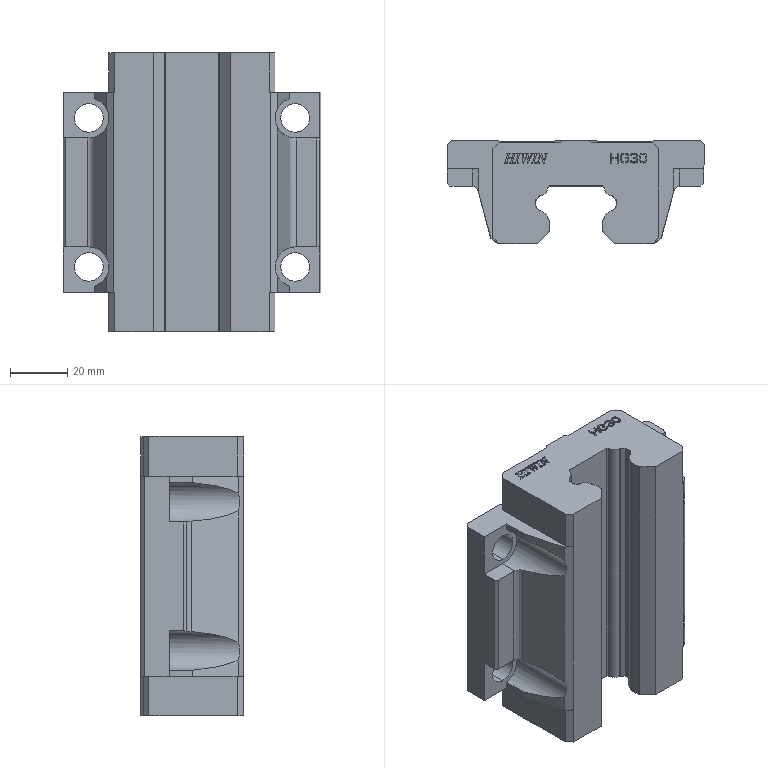Part | STEP file | HGW30 | 1 solid | 414 faces | box 90 x 36 x 97.7 mm | volume 189576 mm3 | plane 320 | spline 60 | cylinder 34 | commonest cylinder face diameters 1.2 x12 10 x8 1.6 x4 5.66 x4 14 x4 5 x2